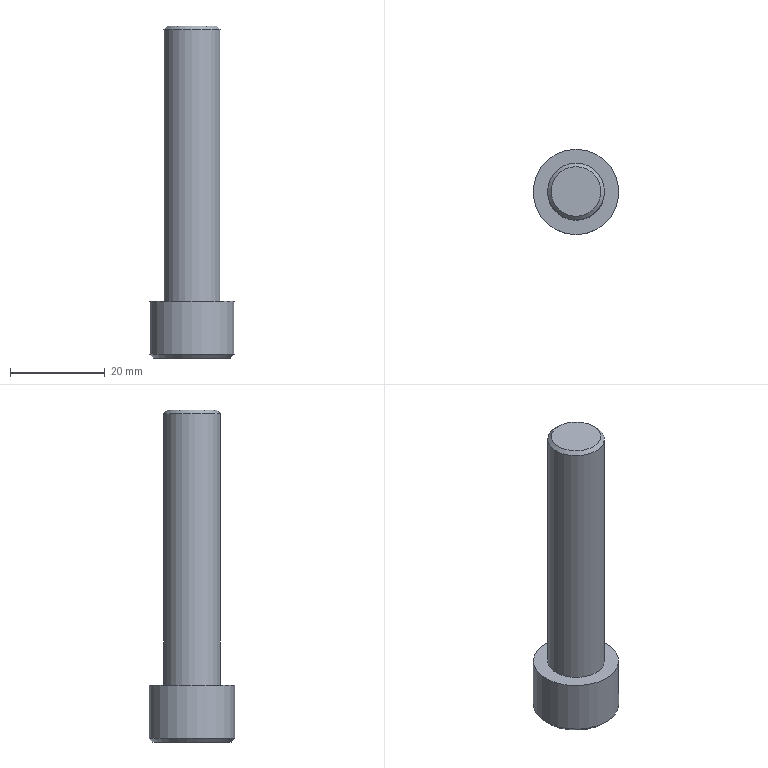Part | STEP file | solid 217 | 1 solid | 14 faces | box 18 x 18 x 70 mm | volume 9155 mm3 | plane 10 | cone 2 | cylinder 2 | commonest cylinder face diameters 12 x1 18 x1